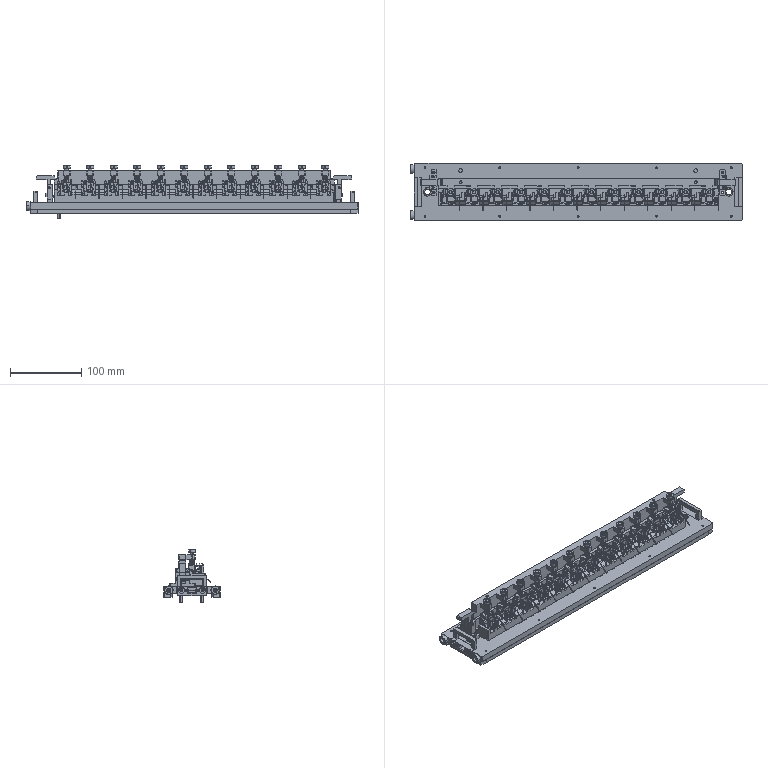Part | NX | features BREP 22 | 93 solids | 8197 faces | volume 699433 mm3 | plane 4961 | cylinder 1806 | spline 1072 | cone 282 | torus 76 | commonest cylinder face diameters 0.5 x468 4 x151 3 x136 0.1 x120 2.5 x96 1 x84